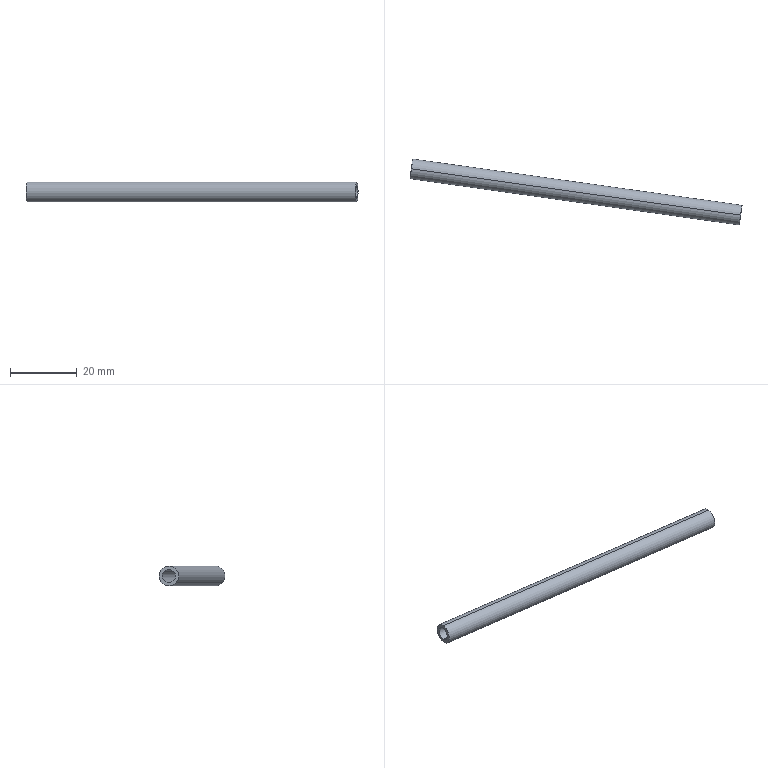Part | SolidWorks | features BaseBody 1 | 1 solid | 6 faces | box 99.862 x 19.859 x 6 mm | volume 1571 mm3 | cylinder 4 | plane 2 | commonest cylinder face diameters 4 x2 6 x2
STEP:
#1=CARTESIAN_POINT('',(-228.468,17.827,-231.5));
#2=VERTEX_POINT('',#1);
#3=CARTESIAN_POINT('',(-228.468,17.827,-235.5));
#4=VERTEX_POINT('',#3);
#5=CARTESIAN_POINT('',(-228.468,17.827,-233.5));
#6=DIRECTION('',(0.9903,-0.1392,0.));
#7=DIRECTION('',(0.,0.,1.));
#8=AXIS2_PLACEMENT_3D('',#5,#6,#7);
#9=CIRCLE('',#8,2.);
#10=EDGE_CURVE('',#2,#4,#9,.T.);
#11=ORIENTED_EDGE('',*,*,#10,.F.);
#12=CARTESIAN_POINT('',(-129.442,3.91,-231.5));
#13=VERTEX_POINT('',#12);
#14=CARTESIAN_POINT('',(-129.442,3.91,-231.5));
#15=DIRECTION('',(0.9903,-0.1392,0.));
#16=VECTOR('',#15,1000.);
#17=LINE('',#14,#16);
#18=EDGE_CURVE('',#2,#13,#17,.T.);
#19=ORIENTED_EDGE('',*,*,#18,.T.);
#20=CARTESIAN_POINT('',(-129.442,3.91,-235.5));
#21=VERTEX_POINT('',#20);
#22=CARTESIAN_POINT('',(-129.442,3.91,-233.5));
#23=DIRECTION('',(0.9903,-0.1392,0.));
#24=DIRECTION('',(0.,0.,-1.));
#25=AXIS2_PLACEMENT_3D('',#22,#23,#24);
#26=CIRCLE('',#25,2.);
#27=EDGE_CURVE('',#13,#21,#26,.T.);
#28=ORIENTED_EDGE('',*,*,#27,.T.);
#29=CARTESIAN_POINT('',(-129.442,3.91,-235.5));
#30=DIRECTION('',(0.9903,-0.1392,0.));
#31=VECTOR('',#30,1000.);
#32=LINE('',#29,#31);
#33=EDGE_CURVE('',#4,#21,#32,.T.);
#34=ORIENTED_EDGE('',*,*,#33,.F.);
#35=EDGE_LOOP('',(#11,#19,#28,#34));
#36=FACE_OUTER_BOUND('',#35,.T.);
#37=CARTESIAN_POINT('',(-129.442,3.91,-233.5));
#38=DIRECTION('',(0.9903,-0.1392,0.));
#39=DIRECTION('',(0.,0.,-1.));
#40=AXIS2_PLACEMENT_3D('',#37,#38,#39);
#41=CYLINDRICAL_SURFACE('',#40,2.);
#42=ADVANCED_FACE('',(#36),#41,.F.);
#43=CARTESIAN_POINT('',(-228.468,17.827,-236.5));
#44=VERTEX_POINT('',#43);
#45=CARTESIAN_POINT('',(-228.468,17.827,-230.5));
#46=VERTEX_POINT('',#45);
#47=CARTESIAN_POINT('',(-228.468,17.827,-233.5));
#48=DIRECTION('',(0.9903,-0.1392,0.));
#49=DIRECTION('',(0.,0.,1.));
#50=AXIS2_PLACEMENT_3D('',#47,#48,#49);
#51=CIRCLE('',#50,3.);
#52=EDGE_CURVE('',#44,#46,#51,.T.);
#53=ORIENTED_EDGE('',*,*,#52,.T.);
#54=CARTESIAN_POINT('',(-129.442,3.91,-230.5));
#55=VERTEX_POINT('',#54);
#56=CARTESIAN_POINT('',(-129.442,3.91,-230.5));
#57=DIRECTION('',(0.9903,-0.1392,0.));
#58=VECTOR('',#57,1000.);
#59=LINE('',#56,#58);
#60=EDGE_CURVE('',#46,#55,#59,.T.);
#61=ORIENTED_EDGE('',*,*,#60,.T.);
#62=CARTESIAN_POINT('',(-129.442,3.91,-236.5));
#63=VERTEX_POINT('',#62);
#64=CARTESIAN_POINT('',(-129.442,3.91,-233.5));
#65=DIRECTION('',(0.9903,-0.1392,0.));
#66=DIRECTION('',(0.,0.,-1.));
#67=AXIS2_PLACEMENT_3D('',#64,#65,#66);
#68=CIRCLE('',#67,3.);
#69=EDGE_CURVE('',#63,#55,#68,.T.);
#70=ORIENTED_EDGE('',*,*,#69,.F.);
#71=CARTESIAN_POINT('',(-129.442,3.91,-236.5));
#72=DIRECTION('',(0.9903,-0.1392,0.));
#73=VECTOR('',#72,1000.);
#74=LINE('',#71,#73);
#75=EDGE_CURVE('',#44,#63,#74,.T.);
#76=ORIENTED_EDGE('',*,*,#75,.F.);
#77=EDGE_LOOP('',(#53,#61,#70,#76));
#78=FACE_OUTER_BOUND('',#77,.T.);
#79=CARTESIAN_POINT('',(-129.442,3.91,-233.5));
#80=DIRECTION('',(0.9903,-0.1392,0.));
#81=DIRECTION('',(0.,0.,-1.));
#82=AXIS2_PLACEMENT_3D('',#79,#80,#81);
#83=CYLINDRICAL_SURFACE('',#82,3.);
#84=ADVANCED_FACE('',(#78),#83,.T.);
#85=ORIENTED_EDGE('',*,*,#60,.F.);
#86=CARTESIAN_POINT('',(-228.468,17.827,-233.5));
#87=DIRECTION('',(0.9903,-0.1392,0.));
#88=DIRECTION('',(0.,0.,1.));
#89=AXIS2_PLACEMENT_3D('',#86,#87,#88);
#90=CIRCLE('',#89,3.);
#91=EDGE_CURVE('',#46,#44,#90,.T.);
#92=ORIENTED_EDGE('',*,*,#91,.T.);
#93=ORIENTED_EDGE('',*,*,#75,.T.);
#94=CARTESIAN_POINT('',(-129.442,3.91,-233.5));
#95=DIRECTION('',(0.9903,-0.1392,0.));
#96=DIRECTION('',(0.,0.,-1.));
#97=AXIS2_PLACEMENT_3D('',#94,#95,#96);
#98=CIRCLE('',#97,3.);
#99=EDGE_CURVE('',#55,#63,#98,.T.);
#100=ORIENTED_EDGE('',*,*,#99,.F.);
#101=EDGE_LOOP('',(#85,#92,#93,#100));
#102=FACE_OUTER_BOUND('',#101,.T.);
#103=CARTESIAN_POINT('',(-129.442,3.91,-233.5));
#104=DIRECTION('',(0.9903,-0.1392,0.));
#105=DIRECTION('',(0.,0.,-1.));
#106=AXIS2_PLACEMENT_3D('',#103,#104,#105);
#107=CYLINDRICAL_SURFACE('',#106,3.);
#108=ADVANCED_FACE('',(#102),#107,.T.);
#109=CARTESIAN_POINT('',(-228.468,17.827,-233.5));
#110=DIRECTION('',(0.9903,-0.1392,0.));
#111=DIRECTION('',(0.,0.,1.));
#112=AXIS2_PLACEMENT_3D('',#109,#110,#111);
#113=CIRCLE('',#112,2.);
#114=EDGE_CURVE('',#4,#2,#113,.T.);
#115=ORIENTED_EDGE('',*,*,#114,.T.);
#116=ORIENTED_EDGE('',*,*,#10,.T.);
#117=EDGE_LOOP('',(#115,#116));
#118=FACE_BOUND('',#117,.T.);
#119=ORIENTED_EDGE('',*,*,#52,.F.);
#120=ORIENTED_EDGE('',*,*,#91,.F.);
#121=EDGE_LOOP('',(#119,#120));
#122=FACE_OUTER_BOUND('',#121,.T.);
#123=CARTESIAN_POINT('',(-228.051,20.798,-233.5));
#124=DIRECTION('',(-0.9903,0.1392,0.));
#125=DIRECTION('',(0.,0.,1.));
#126=AXIS2_PLACEMENT_3D('',#123,#124,#125);
#127=PLANE('',#126);
#128=ADVANCED_FACE('',(#118,#122),#127,.T.);
#129=ORIENTED_EDGE('',*,*,#18,.F.);
#130=ORIENTED_EDGE('',*,*,#114,.F.);
#131=ORIENTED_EDGE('',*,*,#33,.T.);
#132=CARTESIAN_POINT('',(-129.442,3.91,-233.5));
#133=DIRECTION('',(0.9903,-0.1392,0.));
#134=DIRECTION('',(0.,0.,-1.));
#135=AXIS2_PLACEMENT_3D('',#132,#133,#134);
#136=CIRCLE('',#135,2.);
#137=EDGE_CURVE('',#21,#13,#136,.T.);
#138=ORIENTED_EDGE('',*,*,#137,.T.);
#139=EDGE_LOOP('',(#129,#130,#131,#138));
#140=FACE_OUTER_BOUND('',#139,.T.);
#141=CARTESIAN_POINT('',(-129.442,3.91,-233.5));
#142=DIRECTION('',(0.9903,-0.1392,0.));
#143=DIRECTION('',(0.,0.,-1.));
#144=AXIS2_PLACEMENT_3D('',#141,#142,#143);
#145=CYLINDRICAL_SURFACE('',#144,2.);
#146=ADVANCED_FACE('',(#140),#145,.F.);
#147=ORIENTED_EDGE('',*,*,#69,.T.);
#148=ORIENTED_EDGE('',*,*,#99,.T.);
#149=EDGE_LOOP('',(#147,#148));
#150=FACE_OUTER_BOUND('',#149,.T.);
#151=ORIENTED_EDGE('',*,*,#137,.F.);
#152=ORIENTED_EDGE('',*,*,#27,.F.);
#153=EDGE_LOOP('',(#151,#152));
#154=FACE_BOUND('',#153,.T.);
#155=CARTESIAN_POINT('',(-129.163,5.89,-233.5));
#156=DIRECTION('',(0.9903,-0.1392,0.));
#157=DIRECTION('',(0.,0.,-1.));
#158=AXIS2_PLACEMENT_3D('',#155,#156,#157);
#159=PLANE('',#158);
#160=ADVANCED_FACE('',(#150,#154),#159,.T.);
#161=CLOSED_SHELL('',(#42,#84,#108,#128,#146,#160));
#162=MANIFOLD_SOLID_BREP('',#161);
#163=CARTESIAN_POINT('',(0.,0.,0.));
#164=DIRECTION('',(0.,0.,1.));
#165=DIRECTION('',(1.,0.,0.));
#166=AXIS2_PLACEMENT_3D('',#163,#164,#165);
#167=(LENGTH_UNIT()NAMED_UNIT(*)SI_UNIT(.MILLI.,.METRE.));
#168=UNCERTAINTY_MEASURE_WITH_UNIT(LENGTH_MEASURE(0.00001),#167,'','');
#169=(NAMED_UNIT(*)PLANE_ANGLE_UNIT()SI_UNIT($,.RADIAN.));
#170=(NAMED_UNIT(*)SI_UNIT($,.STERADIAN.)SOLID_ANGLE_UNIT());
#171=(GEOMETRIC_REPRESENTATION_CONTEXT(3)GLOBAL_UNCERTAINTY_ASSIGNED_CONTEXT((#168))GLOBAL_UNIT_ASSIGNED_CONTEXT((#167,#169,#170))REPRESENTATION_CONTEXT('',''));
#172=ADVANCED_BREP_SHAPE_REPRESENTATION('',(#162,#166),#171);